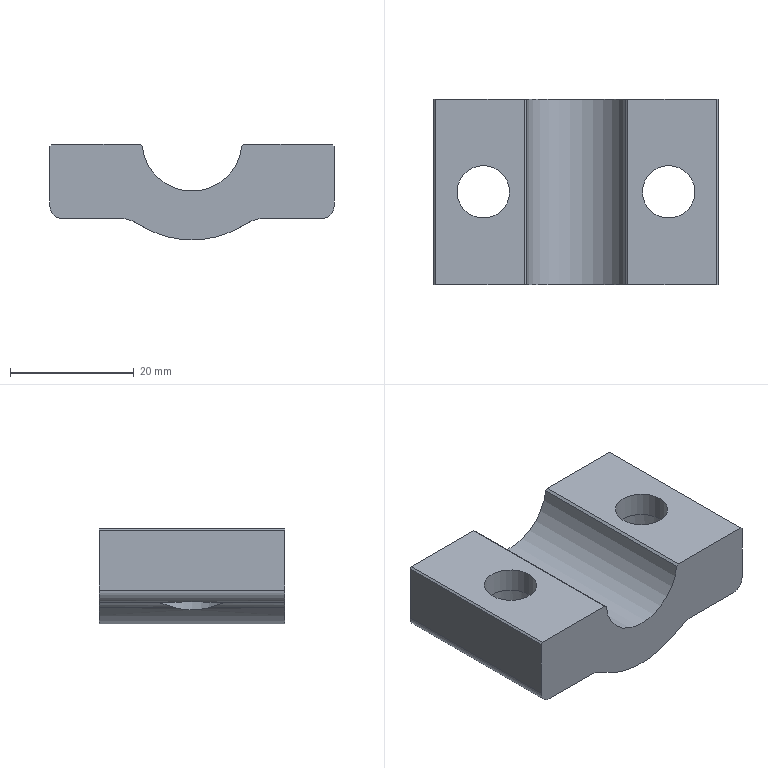NC program | NX | posted with a generic post | part box 46 x 30 x 15.5 mm
Whole program:
N10 G17 G21 G94 G90
(一刀光面_COPY , TOOL : D50R6_1)
N12 T01 M6
N14 G54
N16 G17 G0 G90 X-52.998 Y-1.226 B0. C0. S2000 M3
N18 G43 Z30. H1
N20 Z7.02
N22 G94 G1 Z4.02 F800.
N24 X-48. Y-1.08
N26 X48. Y1.739
N28 X52.998 Y1.886
N30 Z7.02
N32 G0 Z30.
N34 X-52.998 Y-1.226
N36 Z6.04
N38 G1 Z3.04
N40 X-48. Y-1.08
N42 X48. Y1.739
N44 X52.998 Y1.886
N46 Z6.04
N48 G0 Z30.
N50 X-52.998 Y-1.226
N52 Z5.06
N54 G1 Z2.06
N56 X-48. Y-1.08
N58 X48. Y1.739
N60 X52.998 Y1.886
N62 Z5.06
N64 G0 Z30.
N66 X-52.998 Y-1.226
N68 Z4.08
N70 G1 Z1.08
N72 X-48. Y-1.08
N74 X48. Y1.739
N76 X52.998 Y1.886
N78 Z4.08
N80 G0 Z30.
N82 X-52.998 Y-1.226
N84 Z3.1
N86 G1 Z0.1
N88 X-48. Y-1.08
N90 X48. Y1.739
N92 X52.998 Y1.886
N94 Z3.1
N96 G0 Z30.
(一刀光面_COPY_COPY , TOOL : D50R6_1)
N98 X-52.998 Y-1.226
N100 Z3.
N102 G1 Z0.
N104 X-48. Y-1.08
N106 X48. Y1.739
N108 X52.998 Y1.886
N110 Z3.
N112 G0 Z30.
N114 M5
(PLANAR_MILL_COPY_COPY , TOOL : D10点钻)
N116 T04 M6
N118 G54
N120 G17 G0 G90 X4.222 Y9.372 B0. C0. S3000 M3
N122 G43 Z30. H4
N124 Z0.
N126 G94 G1 Z-2. F800.
N128 G3 X7.047 Y9.232 R2.
N130 G2 X8.39 Y9.75 R2.
N132 G1 X22.7
N134 G2 X24.114 Y9.164 R2.
N136 G1 X24.414 Y8.864
N138 G2 X25. Y7.45 R2.
N140 G1 Y-2.25
N142 G2 X21. Y-6.25 R4.
N144 G1 X11.608
N146 G3 X9.95 Y-6.75 R3.
N148 G2 X-9.95 Y-6.75 R18.
N150 G3 X-11.608 Y-6.25 R3.
N152 G1 X-21.
N154 G2 X-25. Y-2.25 R4.
N156 G1 Y7.45
N158 G2 X-24.414 Y8.864 R2.
N160 G1 X-24.114 Y9.164
N162 G2 X-22.7 Y9.75 R2.
N164 G1 X-8.39
N166 G2 X-7.047 Y9.232 R2.
N168 G1 X-6.718 Y8.934
N170 G2 X-6.07 Y7.649 R2.
N172 G3 X6.07 Y7.649 R6.1
N174 G2 X6.718 Y8.934 R2.
N176 G1 X7.047 Y9.232
N178 G3 X7.187 Y12.057 R2.
N180 G1 Z0.
N182 G0 Z30.
N184 M5
N186 M2